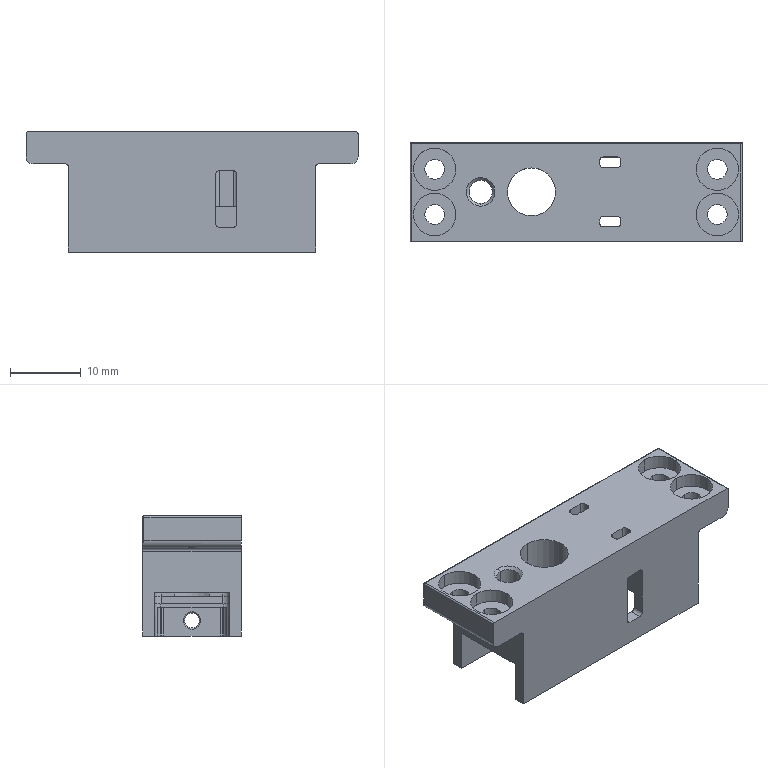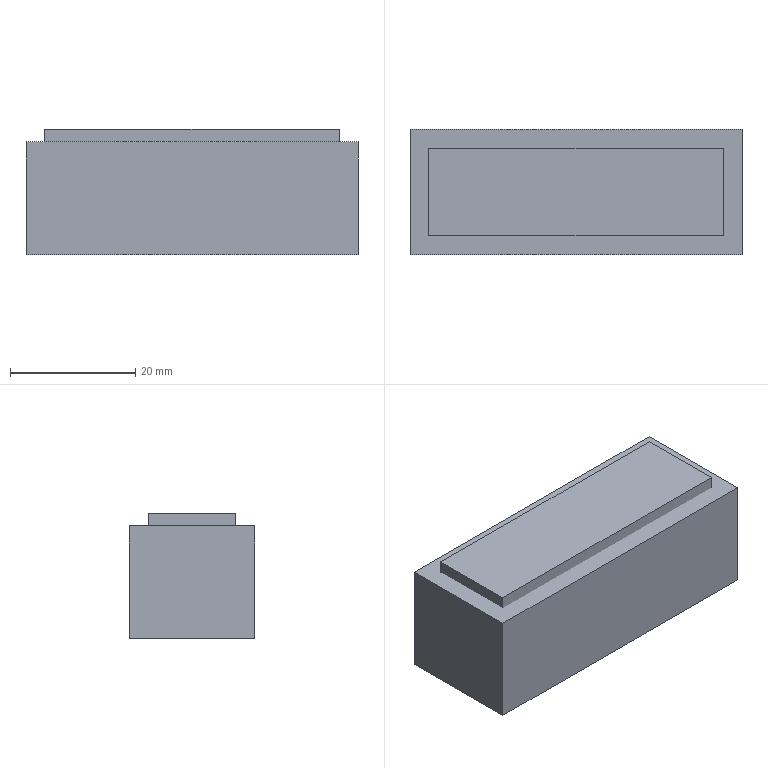CAM job | NX | 3+2 milling, drilling | part box 47 x 14 x 17 mm | stock box 53 x 20 x 20 mm
Tools:
number,name,description,diameter,corner_radius,flute_length,length,flutes
1,D63,Milling Tool-5 Parameters,63.0,0.0,50.0,75.0,2
18,D6A45,Milling Tool-5 Parameters,6.0,0.0,3.0,3.0,2
13,3.4ZT,Drilling Tool,3.3,0.0,35.0,50.0,2
14,M4,Milling Tool-5 Parameters,3.3,0.0,50.0,75.0,2
17,2.8ZT,Drilling Tool,2.8,0.0,35.0,50.0,2
12,7.0ZT,Drilling Tool,6.8,0.0,35.0,50.0,2
19,M8-1,Milling Tool-5 Parameters,6.8,0.0,30.0,30.0,4
3,D10,Milling Tool-5 Parameters,10.0,0.0,50.0,75.0,2
7,D10JING,Milling Tool-5 Parameters,10.0,0.0,50.0,75.0,2
10,D4,Milling Tool-5 Parameters,4.0,0.0,50.0,75.0,2
22,D1,Milling Tool-5 Parameters,1.0,0.0,50.0,75.0,2
20,D2,Milling Tool-5 Parameters,2.0,0.0,50.0,75.0,2
9,D6,Milling Tool-5 Parameters,6.0,0.0,50.0,75.0,2
16,2.1ZT,Drilling Tool,2.05,0.0,35.0,50.0,2
21,M2.5,Milling Tool-5 Parameters,2.05,0.0,30.0,30.0,4
23,R1,Milling Tool-5 Parameters,2.0,1.0,1.0,1.0,2
Operations:
program,operation,operation_type,tool,method,geometry_group,spindle_rpm,surface_speed,feed_per_tooth,feed_cut,feed_plunge,cut_length_mm,path_length_mm,cut_time_min,machine_time_min
1,FLOOR_WALL,VolumeBased25DMillingOperation,D63,METHOD,A,6500.0,1286.0,0.0962,1250.0,100.0,128.0,182.0,0.1024,0.1078
1,DRILLING_COPY_1,Operation,D6A45,METHOD,A,3000.0,56.0,0.0333,200.0,0.0,24.0,179.441,0.12,0.1355
1,DRILLING_COPY_1_COPY,Operation,3.4ZT,METHOD,A,2000.0,20.0,0.0375,150.0,0.0,16.391,92.783,0.1093,0.1169
1,DRILLING_COPY_1_COPY_COPY,Operation,M4,METHOD,A,200.0,2.0,0.0017,0.7,0.0,14.4,88.8,20.571,20.579
1,DRILLING_COPY_1_COPY_COPY_1,Operation,2.8ZT,METHOD,A,2000.0,17.0,0.0375,150.0,0.0,39.365,201.978,0.2624,0.2787
1,DRILLING_COPY_1_COPY_COPY_1_COPY,Operation,7.0ZT,METHOD,A,2000.0,42.0,0.075,300.0,0.0,11.943,83.886,0.0398,0.047
1,DRILLING_COPY_1_COPY_COPY_1_COPY_COPY,Operation,M8-1,METHOD,A,200.0,2.0,0.375,1.0,0.0,8.9,77.8,8.9,8.907
1,ADAPTIVE_MILLING,CavityMilling,D10,METHOD,A,8000.0,251.0,0.2188,3500.0,1000.0,895.182,983.182,0.2579,0.2667
1,ZLEVEL_PROFILE_COPY,ZLevelMilling,D10JING,METHOD,A,8000.0,251.0,0.075,1200.0,100.0,158.669,252.669,0.1322,0.1416
1,HOLE_MILLING,CylinderMilling,D4,METHOD,A,9500.0,119.0,0.0684,1300.0,100.0,195.097,493.897,0.1501,0.18
1,ZLEVEL_PROFILE_COPY_1_COPY,ZLevelMilling,D1,METHOD,A,9500.0,29.0,0.0447,850.0,1000.0,898.364,967.764,1.053,1.06
1,ZLEVEL_PROFILE_COPY_1_COPY_COPY,ZLevelMilling,D1,METHOD,A,9500.0,29.0,0.0447,850.0,1000.0,523.857,588.757,0.6127,0.6192
1,ZLEVEL_PROFILE_COPY_1_COPY_COPY_COPY_COPY_2_COPY,ZLevelMilling,D6A45,METHOD,A,7000.0,131.0,0.0714,1000.0,1000.0,221.368,776.429,0.2214,0.2769
1,刀补7,ZLevelMilling,D10JING,METHOD,A,8000.0,251.0,0.075,1200.0,100.0,63.725,308.617,0.0531,0.0776
2,FLOOR_WALL_COPY,VolumeBased25DMillingOperation,D63,METHOD,B,6500.0,1286.0,0.0962,1250.0,100.0,366.0,754.001,0.2928,0.3316
2,CAVITY_MILL,CavityMilling,D6,METHOD,B,9500.0,179.0,0.1158,2200.0,1000.0,3489.443,3978.287,1.779,1.833
2,HOLE_MILLING_COPY,CylinderMilling,D6,METHOD,B,9500.0,119.0,0.0684,1300.0,100.0,122.867,199.567,0.0945,0.1022
2,CAVITY_MILL_COPY,CavityMilling,D4,METHOD,B,9200.0,115.0,0.0761,1400.0,1000.0,403.318,1103.906,0.321,0.3947
2,FLOOR_WALL_COPY_COPY,VolumeBased25DMillingOperation,D4,METHOD,B,9500.0,298.0,0.0526,1000.0,100.0,558.035,1705.163,0.558,0.6727
2,ZLEVEL_PROFILE_COPY_COPY,ZLevelMilling,D4,METHOD,B,8000.0,251.0,0.075,1200.0,100.0,81.668,319.243,0.0681,0.0918
2,ZLEVEL_PROFILE_COPY_COPY_COPY,ZLevelMilling,D4,METHOD,B,8000.0,251.0,0.1562,2500.0,100.0,704.155,914.23,0.2817,0.3027
2,ZLEVEL_PROFILE_COPY_COPY_COPY_COPY,ZLevelMilling,D4,METHOD,B,8000.0,251.0,0.1562,2500.0,100.0,1258.874,1486,0.5035,0.5263
2,ZLEVEL_PROFILE_COPY_COPY_COPY_COPY_COPY,ZLevelMilling,D4,METHOD,B,8000.0,251.0,0.1562,2500.0,100.0,194.06,277.92,0.0776,0.086
2,CAVITY_MILL_COPY_COPY,CavityMilling,D2,METHOD,B,9200.0,57.0,0.0543,1000.0,1000.0,4042.684,7648.034,4.043,4.422
2,CAVITY_MILL_COPY_COPY_COPY,CavityMilling,D1,METHOD,B,9200.0,28.0,0.0462,850.0,1000.0,3453.981,8738.338,3.875,4.431
2,HOLE_MILLING_COPY_COPY,CylinderMilling,D1,METHOD,B,900.0,2.0,0.5,900.0,100.0,318.911,535.911,0.3543,0.376
2,ZLEVEL_PROFILE_COPY_1_COPY_COPY_COPY_COPY_2_COPY_COPY,ZLevelMilling,D6A45,METHOD,B,7000.0,131.0,0.0714,1000.0,1000.0,166.863,228.863,0.1669,0.1731
2,ZLEVEL_PROFILE_COPY_1_COPY_COPY_COPY_COPY_2_COPY_COPY_COPY_1,ZLevelMilling,R1,METHOD,B,7000.0,131.0,0.0714,1000.0,1000.0,7.89,77.09,0.0079,0.0148
2,ZLEVEL_PROFILE_COPY_1_COPY_COPY_COPY_COPY_2_COPY_COPY_COPY_1_COPY,ZLevelMilling,R1,METHOD,B,7000.0,131.0,0.0714,1000.0,1000.0,18.568,162.981,0.0186,0.033
2,ZLEVEL_PROFILE_COPY_1_COPY_COPY_COPY_COPY_2_COPY_COPY_COPY_1_COPY_COPY,ZLevelMilling,R1,METHOD,B,7000.0,131.0,0.0714,1000.0,1000.0,27.937,258.535,0.0279,0.051
2,ZLEVEL_PROFILE_COPY_1_COPY_COPY_COPY_COPY_2_COPY_COPY_COPY_1_COPY_COPY_COPY,ZLevelMilling,R1,METHOD,B,7000.0,131.0,0.0714,1000.0,1000.0,9.314,81.514,0.0093,0.0165
2,ZLEVEL_PROFILE_COPY_1_COPY_COPY_COPY_COPY_2_COPY_COPY_COPY_1_COPY_COPY_COPY_COPY,ZLevelMilling,R1,METHOD,B,7000.0,131.0,0.0714,1000.0,1000.0,32.839,276.803,0.0328,0.0572
2,刀补10,ZLevelMilling,D4,METHOD,B,8000.0,251.0,0.075,1200.0,100.0,89.397,322.771,0.0745,0.0978
2,刀补10.,ZLevelMilling,D4,METHOD,B,8000.0,251.0,0.075,1200.0,100.0,18.463,99.663,0.0154,0.0235
2,刀补22,ZLevelMilling,D1,METHOD,B,8000.0,251.0,0.075,1200.0,100.0,28.104,171.853,0.0234,0.0378
3,ZLEVEL_PROFILE_COPY_1_COPY_COPY_COPY,ZLevelMilling,D2,METHOD,C,9500.0,29.0,0.0447,850.0,1000.0,1706.123,1776.873,2.003,2.011
3,CAVITY_MILL_COPY_COPY_COPY_COPY,CavityMilling,D1,METHOD,C,9200.0,28.0,0.0462,850.0,1000.0,1052.267,2037.023,1.205,1.319
3,ZLEVEL_PROFILE_COPY_1_COPY_COPY_COPY_COPY_2_COPY_COPY_COPY,ZLevelMilling,D6A45,METHOD,C,7000.0,131.0,0.0714,1000.0,1000.0,15.96,76.96,0.016,0.0221
4,DRILLING_COPY_1_COPY_1,Operation,D6A45,METHOD,D,3000.0,56.0,0.0333,200.0,0.0,4.3,80.6,0.0215,0.0291
4,DRILLING_COPY_1_COPY_COPY_2,Operation,2.1ZT,METHOD,D,2000.0,12.0,0.0375,150.0,0.0,9.416,90.832,0.0628,0.0709
4,DRILLING_COPY_1_COPY_COPY_2_COPY,Operation,M2.5,METHOD,D,200.0,1.0,0.0006,0.45,0.0,7.8,87.6,17.333,17.341